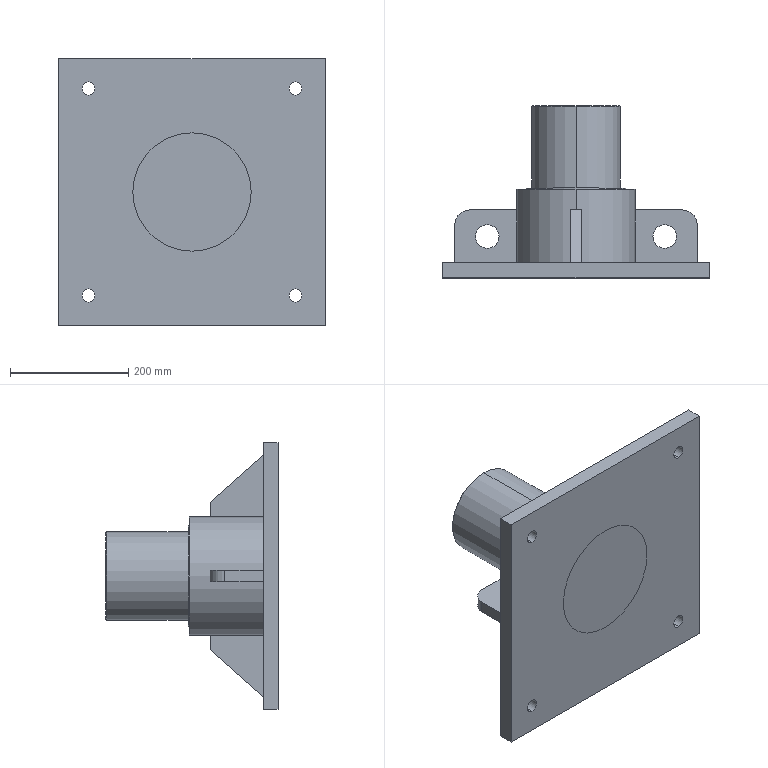Part | SolidWorks | features ICE 7, Fillet 2, 3DProfileFeature 1, Chamfer 1, CirPattern 1, Extrusion 1, HoleWzd 1 | 6 solids | 70 faces | box 450 x 291 x 450 mm | volume 11988612 mm3 | plane 34 | cylinder 28 | cone 8 | commonest cylinder face diameters 22 x8 16.667 x6 40 x4 200 x4 50 x2 150 x2